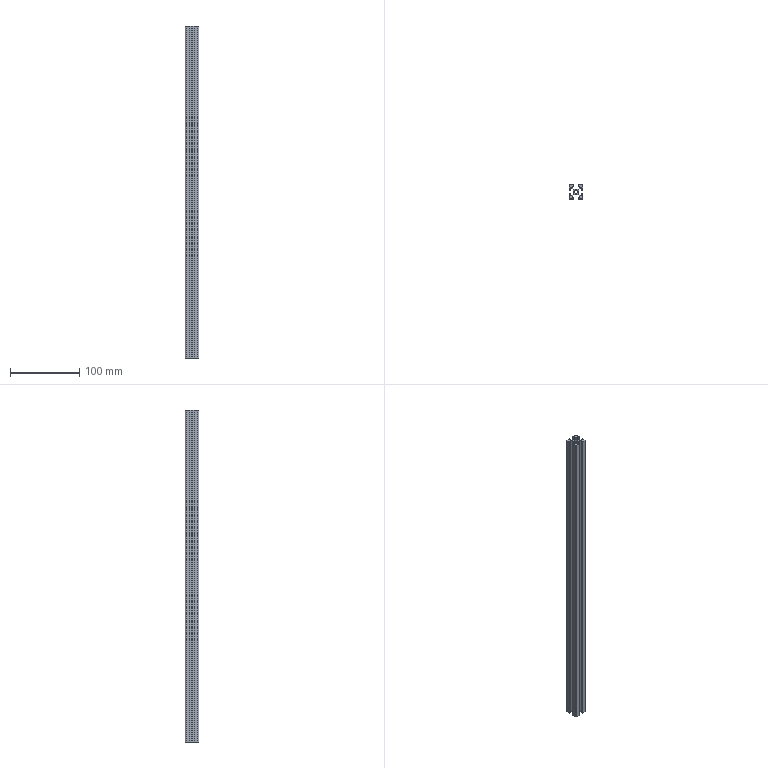Part | STEP file | AOB02-H2020_YHD015 | 1 solid | 80 faces | box 20 x 20 x 480 mm | volume 82868 mm3 | plane 74 | cylinder 6 | commonest cylinder face diameters 3 x4 5 x2